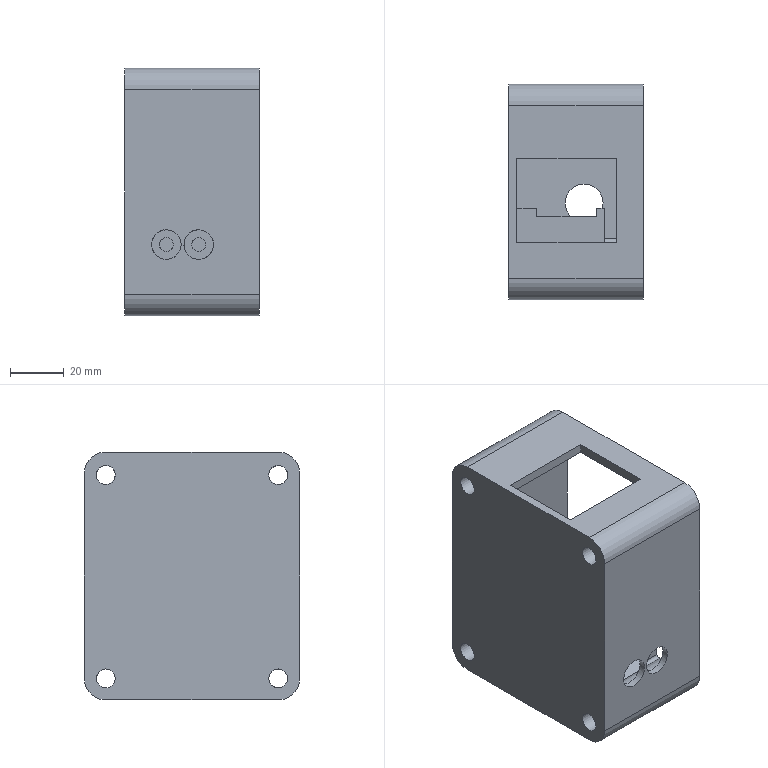NC program | NX | posted by the shop | part box 50 x 80 x 92 mm
Whole program:
%
O1234(5)
(T=7 D6-18-D6-50-3T-rough Z=-18.00 D=6.00 R=0.00 L=50.00)
(T=9 D2-6-D4-50-3T-rough Z=-6.00 D=2.00 R=0.00 L=7.00)
(T=0 D1-10-D4-50-3T Z=-10.00 D=1.00 R=0.00 L=11.00)
G40 G17 G80 G90 G21
M9
M5
G91 G28 Z0.0
M1
N1
(T=11 N=D6-18-D6-50-3T-rough D=1.00 R=0.00 FL=10.00 L=11.00)
(XY-STOCK=0.05)
T11 M6
T9
G0 G90 G54 X-.002 Y-27.801 S4500 M3
G43 H11 Z30.
M8
Z1.
G1 X.063 Y-28.861 Z.981 F800.
X.51 Y-30.015 Z.96
X1.286 Y-30.979 Z.938
X2.318 Y-31.662 Z.917
X3.509 Y-32. Z.895
X4.491 Z.878
X5.682 Y-31.662 Z.856
X6.714 Y-30.979 Z.835
X7.49 Y-30.015 Z.813
X7.937 Y-28.861 Z.791
X8.013 Y-27.625 Z.77
X7.71 Y-26.425 Z.748
X7.219 Y-25.575 Z.731
X6.463 Y-24.81 Z.712
X5.531 Y-24.272 Z.694
X4.491 Y-24. Z.675
X3.509 Z.658
X2.469 Y-24.272 Z.639
X1.537 Y-24.81 Z.62
X.781 Y-25.575 Z.601
X.29 Y-26.425 Z.584
X-.013 Y-27.625 Z.563
X.063 Y-28.861 Z.541
X.51 Y-30.015 Z.519
X1.286 Y-30.979 Z.498
X2.318 Y-31.662 Z.476
X3.509 Y-32. Z.455
X4.491 Z.437
X5.682 Y-31.662 Z.416
X6.714 Y-30.979 Z.394
X7.49 Y-30.015 Z.373
X7.937 Y-28.861 Z.351
X8.013 Y-27.625 Z.329
X7.71 Y-26.425 Z.308
X7.219 Y-25.575 Z.291
X6.463 Y-24.81 Z.272
X5.531 Y-24.272 Z.253
X4.491 Y-24. Z.234
X3.509 Z.217
X2.469 Y-24.272 Z.198
X1.537 Y-24.81 Z.18
X.781 Y-25.575 Z.161
X.29 Y-26.425 Z.144
X-.013 Y-27.625 Z.122
X.063 Y-28.861 Z.101
X.51 Y-30.015 Z.079
X1.286 Y-30.979 Z.057
X2.318 Y-31.662 Z.036
X3.509 Y-32. Z.014
X4.491 Z-.003
X5.682 Y-31.662 Z-.025
X6.714 Y-30.979 Z-.046
X7.49 Y-30.015 Z-.068
X7.937 Y-28.861 Z-.089
X8.013 Y-27.625 Z-.111
X7.71 Y-26.425 Z-.133
X7.219 Y-25.575 Z-.15
X6.463 Y-24.81 Z-.169
X5.531 Y-24.272 Z-.187
X4.491 Y-24. Z-.206
X3.509 Z-.223
X2.469 Y-24.272 Z-.242
X1.537 Y-24.81 Z-.261
X.781 Y-25.575 Z-.28
X.29 Y-26.425 Z-.297
X-.013 Y-27.625 Z-.318
X.063 Y-28.861 Z-.34
X.51 Y-30.015 Z-.361
X1.286 Y-30.979 Z-.383
X2.318 Y-31.662 Z-.405
X3.509 Y-32. Z-.426
X4.491 Z-.443
X5.682 Y-31.662 Z-.465
X6.714 Y-30.979 Z-.487
X7.49 Y-30.015 Z-.508
X7.937 Y-28.861 Z-.53
X8.013 Y-27.625 Z-.551
X7.71 Y-26.425 Z-.573
X7.219 Y-25.575 Z-.59
X6.463 Y-24.81 Z-.609
X5.531 Y-24.272 Z-.628
X4.491 Y-24. Z-.647
X3.509 Z-.664
X2.469 Y-24.272 Z-.682
X1.537 Y-24.81 Z-.701
X.781 Y-25.575 Z-.72
X.29 Y-26.425 Z-.737
X-.013 Y-27.625 Z-.759
X.063 Y-28.861 Z-.78
X.51 Y-30.015 Z-.802
X1.286 Y-30.979 Z-.824
X2.318 Y-31.662 Z-.845
X3.509 Y-32. Z-.867
X4.491 Z-.884
X5.682 Y-31.662 Z-.905
X6.714 Y-30.979 Z-.927
X7.49 Y-30.015 Z-.949
X7.937 Y-28.861 Z-.97
X8.013 Y-27.625 Z-.992
X7.71 Y-26.425 Z-1.014
X7.219 Y-25.575 Z-1.031
X6.463 Y-24.81 Z-1.049
X5.531 Y-24.272 Z-1.068
X4.491 Y-24. Z-1.087
X3.509 Z-1.104
X2.469 Y-24.272 Z-1.123
X1.537 Y-24.81 Z-1.142
X.781 Y-25.575 Z-1.16
X.29 Y-26.425 Z-1.178
X-.013 Y-27.625 Z-1.199
X.063 Y-28.861 Z-1.221
X.51 Y-30.015 Z-1.242
X1.286 Y-30.979 Z-1.264
X2.318 Y-31.662 Z-1.286
X3.509 Y-32. Z-1.307
X4.491 Z-1.324
X5.682 Y-31.662 Z-1.346
X6.714 Y-30.979 Z-1.368
X7.49 Y-30.015 Z-1.389
X7.937 Y-28.861 Z-1.411
X8.013 Y-27.625 Z-1.432
X7.71 Y-26.425 Z-1.454
X7.219 Y-25.575 Z-1.471
X6.463 Y-24.81 Z-1.49
X5.531 Y-24.272 Z-1.509
X4.491 Y-24. Z-1.527
X3.509 Z-1.545
X2.469 Y-24.272 Z-1.563
X1.537 Y-24.81 Z-1.582
X.781 Y-25.575 Z-1.601
X.29 Y-26.425 Z-1.618
X-.013 Y-27.625 Z-1.64
X.063 Y-28.861 Z-1.661
X.51 Y-30.015 Z-1.683
X1.286 Y-30.979 Z-1.704
X2.318 Y-31.662 Z-1.726
X3.509 Y-32. Z-1.748
X4.491 Z-1.765
X5.682 Y-31.662 Z-1.786
X6.714 Y-30.979 Z-1.808
X7.49 Y-30.015 Z-1.83
X7.937 Y-28.861 Z-1.851
X8.013 Y-27.625 Z-1.873
X7.71 Y-26.425 Z-1.894
X7.219 Y-25.575 Z-1.912
X6.463 Y-24.81 Z-1.93
X5.531 Y-24.272 Z-1.949
X4.491 Y-24. Z-1.968
X3.509 Z-1.985
X2.469 Y-24.272 Z-2.004
X1.537 Y-24.81 Z-2.023
X.781 Y-25.575 Z-2.041
X.29 Y-26.425 Z-2.058
X-.013 Y-27.625 Z-2.08
X.063 Y-28.861 Z-2.102
X.51 Y-30.015 Z-2.123
X1.286 Y-30.979 Z-2.145
X2.318 Y-31.662 Z-2.166
X3.509 Y-32. Z-2.188
X4.491 Z-2.205
X5.682 Y-31.662 Z-2.227
X6.714 Y-30.979 Z-2.248
X7.49 Y-30.015 Z-2.27
X7.937 Y-28.861 Z-2.292
X8.013 Y-27.625 Z-2.313
X7.71 Y-26.425 Z-2.335
X7.219 Y-25.575 Z-2.352
X6.463 Y-24.81 Z-2.371
X5.531 Y-24.272 Z-2.39
X4.491 Y-24. Z-2.408
X3.509 Z-2.425
X2.469 Y-24.272 Z-2.444
X1.537 Y-24.81 Z-2.463
X.781 Y-25.575 Z-2.482
X.29 Y-26.425 Z-2.499
X-.013 Y-27.625 Z-2.521
X.063 Y-28.861 Z-2.542
X.51 Y-30.015 Z-2.564
X1.286 Y-30.979 Z-2.585
X2.318 Y-31.662 Z-2.607
X3.509 Y-32. Z-2.629
X4.491 Z-2.646
X5.682 Y-31.662 Z-2.667
X6.714 Y-30.979 Z-2.689
X7.49 Y-30.015 Z-2.71
X7.937 Y-28.861 Z-2.732
X8.013 Y-27.625 Z-2.754
X7.71 Y-26.425 Z-2.775
X7.219 Y-25.575 Z-2.792
X6.463 Y-24.81 Z-2.811
X5.531 Y-24.272 Z-2.83
X4.491 Y-24. Z-2.849
X3.509 Z-2.866
X2.469 Y-24.272 Z-2.885
X1.537 Y-24.81 Z-2.903
X.781 Y-25.575 Z-2.922
X.29 Y-26.425 Z-2.939
X-.013 Y-27.625 Z-2.961
X.063 Y-28.861 Z-2.983
X.51 Y-30.015 Z-3.004
X1.286 Y-30.979 Z-3.026
X2.318 Y-31.662 Z-3.047
X3.509 Y-32. Z-3.069
X4.491 Z-3.086
X5.682 Y-31.662 Z-3.108
X6.714 Y-30.979 Z-3.129
X7.49 Y-30.015 Z-3.151
X7.937 Y-28.861 Z-3.173
X8.013 Y-27.625 Z-3.194
X7.71 Y-26.425 Z-3.216
X7.219 Y-25.575 Z-3.233
X6.463 Y-24.81 Z-3.252
X5.531 Y-24.272 Z-3.27
X4.491 Y-24. Z-3.289
X3.509 Z-3.306
X2.469 Y-24.272 Z-3.325
X1.537 Y-24.81 Z-3.344
X.781 Y-25.575 Z-3.363
X.29 Y-26.425 Z-3.38
X-.013 Y-27.625 Z-3.401
X.063 Y-28.861 Z-3.423
X.51 Y-30.015 Z-3.445
X1.286 Y-30.979 Z-3.466
X2.318 Y-31.662 Z-3.488
X3.509 Y-32. Z-3.509
X4.491 Z-3.527
X5.682 Y-31.662 Z-3.548
X6.714 Y-30.979 Z-3.57
X7.49 Y-30.015 Z-3.591
X7.937 Y-28.861 Z-3.613
X8.013 Y-27.625 Z-3.635
X7.71 Y-26.425 Z-3.656
X7.219 Y-25.575 Z-3.673
X6.463 Y-24.81 Z-3.692
X5.531 Y-24.272 Z-3.711
X4.491 Y-24. Z-3.73
X3.509 Z-3.747
X2.469 Y-24.272 Z-3.766
X1.537 Y-24.81 Z-3.784
X.781 Y-25.575 Z-3.803
X.29 Y-26.425 Z-3.82
X-.013 Y-27.625 Z-3.842
X.063 Y-28.861 Z-3.863
X.51 Y-30.015 Z-3.885
X1.286 Y-30.979 Z-3.907
X2.318 Y-31.662 Z-3.928
X3.509 Y-32. Z-3.95
X4.491 Z-3.967
X5.682 Y-31.662 Z-3.989
X6.714 Y-30.979 Z-4.01
X7.49 Y-30.015 Z-4.032
X7.937 Y-28.861 Z-4.053
X8.013 Y-27.625 Z-4.075
X7.71 Y-26.425 Z-4.097
X7.219 Y-25.575 Z-4.114
X6.463 Y-24.81 Z-4.133
X5.531 Y-24.272 Z-4.151
X4.491 Y-24. Z-4.17
X3.509 Z-4.187
X2.469 Y-24.272 Z-4.206
X1.537 Y-24.81 Z-4.225
X.781 Y-25.575 Z-4.244
X.29 Y-26.425 Z-4.261
X-.013 Y-27.625 Z-4.282
X.063 Y-28.861 Z-4.304
X.51 Y-30.015 Z-4.326
X1.286 Y-30.979 Z-4.347
X2.318 Y-31.662 Z-4.369
X3.509 Y-32. Z-4.39
X4.491 Z-4.407
X5.682 Y-31.662 Z-4.429
X6.714 Y-30.979 Z-4.451
X7.49 Y-30.015 Z-4.472
X7.937 Y-28.861 Z-4.494
X8.013 Y-27.625 Z-4.515
X7.71 Y-26.425 Z-4.537
X7.219 Y-25.575 Z-4.554
X6.463 Y-24.81 Z-4.573
X5.531 Y-24.272 Z-4.592
X4.491 Y-24. Z-4.611
X3.509 Z-4.628
X2.469 Y-24.272 Z-4.646
X1.537 Y-24.81 Z-4.665
X.781 Y-25.575 Z-4.684
X.29 Y-26.425 Z-4.701
X-.013 Y-27.625 Z-4.723
X.063 Y-28.861 Z-4.744
X.51 Y-30.015 Z-4.766
X1.286 Y-30.979 Z-4.788
X2.318 Y-31.662 Z-4.809
X3.509 Y-32. Z-4.831
X4.491 Z-4.848
X5.682 Y-31.662 Z-4.87
X6.714 Y-30.979 Z-4.891
X7.49 Y-30.015 Z-4.913
X7.937 Y-28.861 Z-4.934
X8.013 Y-27.625 Z-4.956
X7.71 Y-26.425 Z-4.978
X7.219 Y-25.575 Z-4.995
X6.463 Y-24.81 Z-5.013
X5.531 Y-24.272 Z-5.032
X4.491 Y-24. Z-5.051
X3.509 Z-5.068
X2.469 Y-24.272 Z-5.087
X1.537 Y-24.81 Z-5.106
X.781 Y-25.575 Z-5.124
X.29 Y-26.425 Z-5.142
X-.013 Y-27.625 Z-5.163
X.063 Y-28.861 Z-5.185
X.51 Y-30.015 Z-5.206
X1.286 Y-30.979 Z-5.228
X2.318 Y-31.662 Z-5.25
X3.509 Y-32. Z-5.271
X4.491 Z-5.288
X5.682 Y-31.662 Z-5.31
X6.714 Y-30.979 Z-5.332
X7.49 Y-30.015 Z-5.353
X7.937 Y-28.861 Z-5.375
X8.013 Y-27.625 Z-5.396
X7.71 Y-26.425 Z-5.418
X7.219 Y-25.575 Z-5.435
X6.463 Y-24.81 Z-5.454
X5.531 Y-24.272 Z-5.473
X4.491 Y-24. Z-5.491
X4. Z-5.5
G3 I0.0 J-4.
G1 Z-4.5
G0 Z30.
G0 X9.65 Y-28.654 S4500 M3
M8
Z1.
G1 Y-24.738 Z.932 F800.
X4. Y-21.476 Z.818
X-1.65 Y-24.738 Z.704
Y-31.262 Z.59
X4. Y-34.524 Z.476
X9.65 Y-31.262 Z.362
Y-24.738 Z.248
X4. Y-21.476 Z.134
X-1.65 Y-24.738 Z.021
Y-31.262 Z-.093
X4. Y-34.524 Z-.207
X9.65 Y-31.262 Z-.321
Y-24.738 Z-.435
X4. Y-21.476 Z-.549
X-1.65 Y-24.738 Z-.663
Y-31.262 Z-.777
X4. Y-34.524 Z-.89
X9.65 Y-31.262 Z-1.004
Y-24.738 Z-1.118
X4. Y-21.476 Z-1.232
X-1.65 Y-24.738 Z-1.346
Y-31.262 Z-1.46
X4. Y-34.524 Z-1.574
X9.65 Y-31.262 Z-1.688
Y-24.738 Z-1.801
X4. Y-21.476 Z-1.915
X-1.65 Y-24.738 Z-2.029
Y-31.262 Z-2.143
X1.175 Y-32.893 Z-2.2
X4. Y-34.524
X9.65 Y-31.262
Y-24.738
X4. Y-21.476
X-1.65 Y-24.738
Y-31.262
X1.175 Y-32.893
Z-1.2
G0 Z30.
G0 X5. Y-25.119 S4500 M3
M8
Z-3.5
G1 Z-5.5 F600.
Y-24.95
G3 X4. Y-23.95 I-1. J0.0
I0.0 J-4.05
X3. Y-24.95 I0.0 J-1.
G1 Y-25.119
Z-3.5
G0 Z30.
M9
M5
G91 G28 Z0.0
M1
N2
(T=9 N=D2-6-D4-50-3T-rough D=2.00 R=0.00 FL=6.00 L=7.00)
(XY-STOCK=0.00)
T9 M6
T10
G0 G90 G54 X11.7 Y-30.145 S4500 M3
G43 H09 Z30.
M8
Z1.
G1 Y-23.554 Z.942 F800.
X4. Y-19.109 Z.865
X-3.7 Y-23.554 Z.787
Y-32.446 Z.71
X4. Y-36.891 Z.632
X11.7 Y-32.446 Z.555
Y-23.554 Z.477
X4. Y-19.109 Z.399
X-3.7 Y-23.554 Z.322
Y-32.446 Z.244
X4. Y-36.891 Z.167
X11.7 Y-32.446 Z.089
Y-23.554 Z.011
X4. Y-19.109 Z-.066
X-3.7 Y-23.554 Z-.144
Y-32.446 Z-.221
X4. Y-36.891 Z-.299
X11.7 Y-32.446 Z-.377
Y-23.554 Z-.454
X4. Y-19.109 Z-.532
X-3.7 Y-23.554 Z-.609
Y-32.446 Z-.687
X4. Y-36.891 Z-.765
X11.7 Y-32.446 Z-.842
Y-23.554 Z-.92
X4. Y-19.109 Z-.997
X-3.7 Y-23.554 Z-1.075
Y-32.446 Z-1.153
X4. Y-36.891 Z-1.23
X11.7 Y-32.446 Z-1.308
Y-23.554 Z-1.385
X4. Y-19.109 Z-1.463
X-3.7 Y-23.554 Z-1.54
Y-32.446 Z-1.618
X4. Y-36.891 Z-1.696
X11.7 Y-32.446 Z-1.773
Y-23.554 Z-1.851
X4. Y-19.109 Z-1.928
X-3.7 Y-23.554 Z-2.006
Y-32.446 Z-2.084
X4. Y-36.891 Z-2.161
X7.85 Y-34.668 Z-2.2
X11.7 Y-32.446
Y-23.554
X4. Y-19.109
X-3.7 Y-23.554
Y-32.446
X4. Y-36.891
X7.85 Y-34.668
Z-1.2
G0 Z30.
M9
M5
G91 G28 Z0.0
M1
N3
(T=10 N=D1-10-D4-50-3T D=1.00 R=0.00 FL=10.00 L=11.00)
(XY-STOCK=0.05)
T10 M6
T11
G0 G90 G54 X.404 Y-35.335 S4500 M3
G43 H10 Z30.
M8
Z1.
G1 X4. Y-37.411 Z.978 F800.
X12.15 Y-32.705 Z.929
Y-23.295 Z.88
X4. Y-18.589 Z.83
X-4.15 Y-23.295 Z.781
Y-32.705 Z.732
X4. Y-37.411 Z.683
X12.15 Y-32.705 Z.633
Y-23.295 Z.584
X4. Y-18.589 Z.535
X-4.15 Y-23.295 Z.486
Y-32.705 Z.436
X4. Y-37.411 Z.387
X12.15 Y-32.705 Z.338
Y-23.295 Z.288
X4. Y-18.589 Z.239
X-4.15 Y-23.295 Z.19
Y-32.705 Z.141
X4. Y-37.411 Z.091
X12.15 Y-32.705 Z.042
Y-23.295 Z-.007
X4. Y-18.589 Z-.057
X-4.15 Y-23.295 Z-.106
Y-32.705 Z-.155
X4. Y-37.411 Z-.204
X12.15 Y-32.705 Z-.254
Y-23.295 Z-.303
X4. Y-18.589 Z-.352
X-4.15 Y-23.295 Z-.401
Y-32.705 Z-.451
X4. Y-37.411 Z-.5
X12.15 Y-32.705 Z-.549
Y-23.295 Z-.599
X4. Y-18.589 Z-.648
X-4.15 Y-23.295 Z-.697
Y-32.705 Z-.746
X4. Y-37.411 Z-.796
X12.15 Y-32.705 Z-.845
Y-23.295 Z-.894
X4. Y-18.589 Z-.943
X-4.15 Y-23.295 Z-.993
Y-32.705 Z-1.042
X4. Y-37.411 Z-1.091
X12.15 Y-32.705 Z-1.141
Y-23.295 Z-1.19
X4. Y-18.589 Z-1.239
X-4.15 Y-23.295 Z-1.288
Y-32.705 Z-1.338
X4. Y-37.411 Z-1.387
X12.15 Y-32.705 Z-1.436
Y-23.295 Z-1.486
X4. Y-18.589 Z-1.535
X-4.15 Y-23.295 Z-1.584
Y-32.705 Z-1.633
X4. Y-37.411 Z-1.683
X12.15 Y-32.705 Z-1.732
Y-23.295 Z-1.781
X4. Y-18.589 Z-1.83
X-4.15 Y-23.295 Z-1.88
Y-32.705 Z-1.929
X4. Y-37.411 Z-1.978
X12.15 Y-32.705 Z-2.028
Y-23.295 Z-2.077
X4. Y-18.589 Z-2.126
X-4.15 Y-23.295 Z-2.175
Y-28. Z-2.2
Y-32.705
X4. Y-37.411
X12.15 Y-32.705
Y-23.295
X4. Y-18.589
X-4.15 Y-23.295
Y-28.
Z-1.2
G0 Z30.
M9
M5
G91 G28 Z0.0
G28 Y0.
M30
%